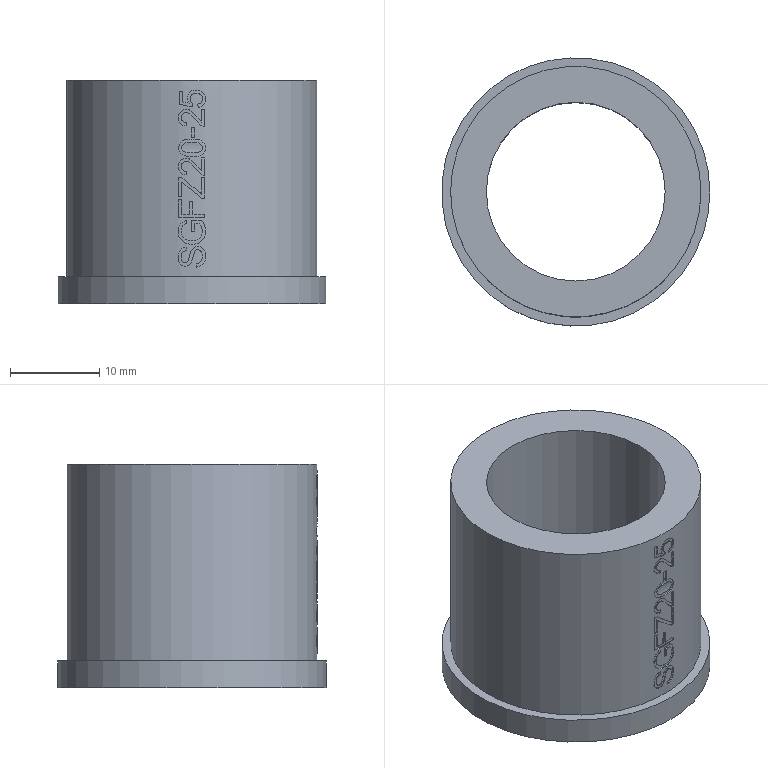Part | NX | features SGFZ20-25_1 2 | 1 solid | 143 faces | box 30 x 30 x 25 mm | volume 7808 mm3 | plane 82 | cylinder 58 | torus 3 | commonest cylinder face diameters 27.8 x9 20 x4 1.13 x2 1.721 x2 1.843 x2 1.919 x2